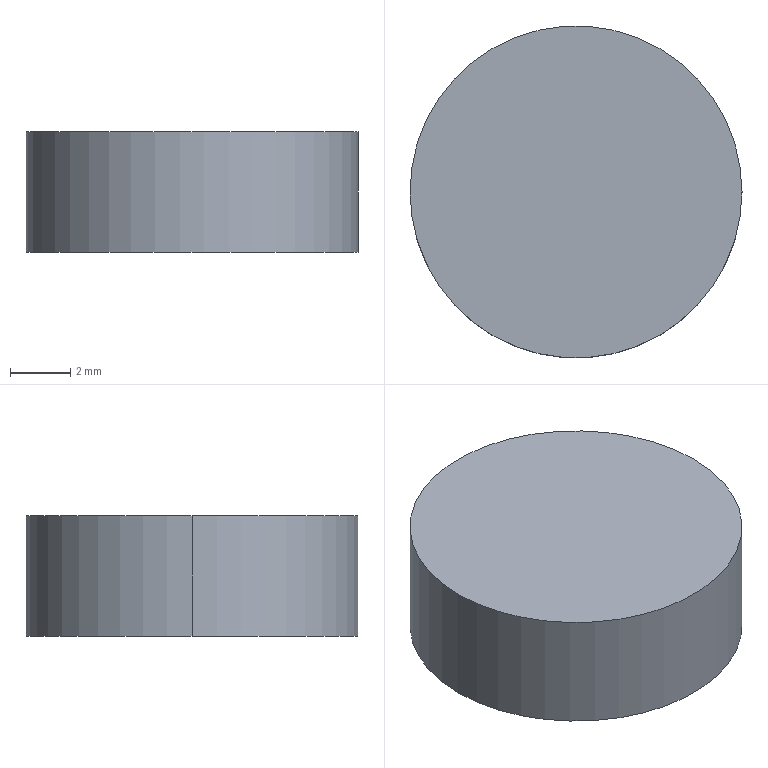Part | STEP file | 1_id258_x_t | 1 solid | 4 faces | box 11 x 11 x 4 mm | volume 380.137 mm3 | plane 2 | cylinder 2 | commonest cylinder face diameters 11 x2
STEP:
#1=CARTESIAN_POINT('',(0.,0.,0.));
#2=DIRECTION('',(0.,0.,1.));
#3=DIRECTION('',(1.,0.,0.));
#4=AXIS2_PLACEMENT_3D('',#1,#2,#3);
#5=CARTESIAN_POINT('',(201.65,177.5,39.075));
#6=VERTEX_POINT('',#5);
#7=CARTESIAN_POINT('',(212.65,177.5,39.075));
#8=VERTEX_POINT('',#7);
#9=CARTESIAN_POINT('',(207.15,177.5,39.075));
#10=DIRECTION('',(0.,0.,1.));
#11=DIRECTION('',(-1.,0.,0.));
#12=AXIS2_PLACEMENT_3D('',#9,#10,#11);
#13=CIRCLE('',#12,5.5);
#14=CARTESIAN_POINT('',(274.812,177.5,39.075));
#15=DIRECTION('',(0.,0.,-1.));
#16=DIRECTION('',(-1.,0.,0.));
#17=AXIS2_PLACEMENT_3D('',#14,#15,#16);
#18=PLANE('',#17);
#19=CARTESIAN_POINT('',(73.162,0.));
#20=CARTESIAN_POINT('',(73.162,-9.526));
#21=CARTESIAN_POINT('',(64.912,-4.763));
#22=CARTESIAN_POINT('',(56.663,0.));
#23=CARTESIAN_POINT('',(64.912,4.763));
#24=CARTESIAN_POINT('',(73.162,9.526));
#25=CARTESIAN_POINT('',(73.162,0.));
#26=(BOUNDED_CURVE()B_SPLINE_CURVE(2,(#19,#20,#21,#22,#23,#24,#25),.UNSPECIFIED.,.T.,.F.)B_SPLINE_CURVE_WITH_KNOTS((1,2,2,2,2,1),(-2.094,0.,2.094,4.189,6.283,8.378),.UNSPECIFIED.)CURVE()GEOMETRIC_REPRESENTATION_ITEM()RATIONAL_B_SPLINE_CURVE((1.,0.5,1.,0.5,1.,0.5,1.))REPRESENTATION_ITEM(''));
#27=(GEOMETRIC_REPRESENTATION_CONTEXT(2)PARAMETRIC_REPRESENTATION_CONTEXT()REPRESENTATION_CONTEXT('',''));
#28=DEFINITIONAL_REPRESENTATION('',(#26),#27);
#29=PCURVE('',#18,#28);
#30=CARTESIAN_POINT('',(207.15,177.5,43.075));
#31=DIRECTION('',(0.,0.,-1.));
#32=DIRECTION('',(-1.,0.,0.));
#33=AXIS2_PLACEMENT_3D('',#30,#31,#32);
#34=CYLINDRICAL_SURFACE('',#33,5.5);
#35=CARTESIAN_POINT('',(6.283,4.));
#36=DIRECTION('',(-1.,0.));
#37=VECTOR('',#36,1.);
#38=LINE('',#35,#37);
#39=(GEOMETRIC_REPRESENTATION_CONTEXT(2)PARAMETRIC_REPRESENTATION_CONTEXT()REPRESENTATION_CONTEXT('',''));
#40=DEFINITIONAL_REPRESENTATION('',(#38),#39);
#41=PCURVE('',#34,#40);
#42=SURFACE_CURVE('',#13,(#29,#41),.PCURVE_S1.);
#43=EDGE_CURVE('',#6,#8,#42,.T.);
#44=ORIENTED_EDGE('',*,*,#43,.F.);
#45=CARTESIAN_POINT('',(207.15,177.5,39.075));
#46=DIRECTION('',(0.,0.,1.));
#47=DIRECTION('',(-1.,0.,0.));
#48=AXIS2_PLACEMENT_3D('',#45,#46,#47);
#49=CIRCLE('',#48,5.5);
#50=CARTESIAN_POINT('',(73.162,0.));
#51=CARTESIAN_POINT('',(73.162,-9.526));
#52=CARTESIAN_POINT('',(64.912,-4.763));
#53=CARTESIAN_POINT('',(56.663,0.));
#54=CARTESIAN_POINT('',(64.912,4.763));
#55=CARTESIAN_POINT('',(73.162,9.526));
#56=CARTESIAN_POINT('',(73.162,0.));
#57=(BOUNDED_CURVE()B_SPLINE_CURVE(2,(#50,#51,#52,#53,#54,#55,#56),.UNSPECIFIED.,.T.,.F.)B_SPLINE_CURVE_WITH_KNOTS((1,2,2,2,2,1),(-2.094,0.,2.094,4.189,6.283,8.378),.UNSPECIFIED.)CURVE()GEOMETRIC_REPRESENTATION_ITEM()RATIONAL_B_SPLINE_CURVE((1.,0.5,1.,0.5,1.,0.5,1.))REPRESENTATION_ITEM(''));
#58=(GEOMETRIC_REPRESENTATION_CONTEXT(2)PARAMETRIC_REPRESENTATION_CONTEXT()REPRESENTATION_CONTEXT('',''));
#59=DEFINITIONAL_REPRESENTATION('',(#57),#58);
#60=PCURVE('',#18,#59);
#61=CARTESIAN_POINT('',(207.15,177.5,43.075));
#62=DIRECTION('',(0.,0.,-1.));
#63=DIRECTION('',(-1.,0.,0.));
#64=AXIS2_PLACEMENT_3D('',#61,#62,#63);
#65=CYLINDRICAL_SURFACE('',#64,5.5);
#66=CARTESIAN_POINT('',(6.283,4.));
#67=DIRECTION('',(-1.,0.));
#68=VECTOR('',#67,1.);
#69=LINE('',#66,#68);
#70=(GEOMETRIC_REPRESENTATION_CONTEXT(2)PARAMETRIC_REPRESENTATION_CONTEXT()REPRESENTATION_CONTEXT('',''));
#71=DEFINITIONAL_REPRESENTATION('',(#69),#70);
#72=PCURVE('',#65,#71);
#73=SURFACE_CURVE('',#49,(#60,#72),.PCURVE_S1.);
#74=EDGE_CURVE('',#8,#6,#73,.T.);
#75=ORIENTED_EDGE('',*,*,#74,.F.);
#76=EDGE_LOOP('',(#44,#75));
#77=FACE_BOUND('',#76,.T.);
#78=ADVANCED_FACE('',(#77),#18,.T.);
#79=CARTESIAN_POINT('',(201.65,177.5,43.075));
#80=VERTEX_POINT('',#79);
#81=CARTESIAN_POINT('',(212.65,177.5,43.075));
#82=VERTEX_POINT('',#81);
#83=CARTESIAN_POINT('',(207.15,177.5,43.075));
#84=DIRECTION('',(0.,0.,1.));
#85=DIRECTION('',(-1.,0.,0.));
#86=AXIS2_PLACEMENT_3D('',#83,#84,#85);
#87=CIRCLE('',#86,5.5);
#88=CARTESIAN_POINT('',(207.15,177.5,43.075));
#89=DIRECTION('',(0.,0.,1.));
#90=DIRECTION('',(1.,0.,0.));
#91=AXIS2_PLACEMENT_3D('',#88,#89,#90);
#92=PLANE('',#91);
#93=CARTESIAN_POINT('',(0.,0.));
#94=DIRECTION('',(-1.,0.));
#95=AXIS2_PLACEMENT_2D('',#93,#94);
#96=CIRCLE('',#95,5.5);
#97=(GEOMETRIC_REPRESENTATION_CONTEXT(2)PARAMETRIC_REPRESENTATION_CONTEXT()REPRESENTATION_CONTEXT('',''));
#98=DEFINITIONAL_REPRESENTATION('',(#96),#97);
#99=PCURVE('',#92,#98);
#100=CARTESIAN_POINT('',(6.283,0.));
#101=DIRECTION('',(-1.,0.));
#102=VECTOR('',#101,1.);
#103=LINE('',#100,#102);
#104=(GEOMETRIC_REPRESENTATION_CONTEXT(2)PARAMETRIC_REPRESENTATION_CONTEXT()REPRESENTATION_CONTEXT('',''));
#105=DEFINITIONAL_REPRESENTATION('',(#103),#104);
#106=PCURVE('',#34,#105);
#107=SURFACE_CURVE('',#87,(#99,#106),.PCURVE_S1.);
#108=EDGE_CURVE('',#80,#82,#107,.T.);
#109=ORIENTED_EDGE('',*,*,#108,.T.);
#110=CARTESIAN_POINT('',(207.15,177.5,43.075));
#111=DIRECTION('',(0.,0.,1.));
#112=DIRECTION('',(1.,0.,0.));
#113=AXIS2_PLACEMENT_3D('',#110,#111,#112);
#114=CIRCLE('',#113,5.5);
#115=CARTESIAN_POINT('',(0.,0.));
#116=DIRECTION('',(1.,0.));
#117=AXIS2_PLACEMENT_2D('',#115,#116);
#118=CIRCLE('',#117,5.5);
#119=(GEOMETRIC_REPRESENTATION_CONTEXT(2)PARAMETRIC_REPRESENTATION_CONTEXT()REPRESENTATION_CONTEXT('',''));
#120=DEFINITIONAL_REPRESENTATION('',(#118),#119);
#121=PCURVE('',#92,#120);
#122=CARTESIAN_POINT('',(3.142,0.));
#123=DIRECTION('',(-1.,0.));
#124=VECTOR('',#123,1.);
#125=LINE('',#122,#124);
#126=(GEOMETRIC_REPRESENTATION_CONTEXT(2)PARAMETRIC_REPRESENTATION_CONTEXT()REPRESENTATION_CONTEXT('',''));
#127=DEFINITIONAL_REPRESENTATION('',(#125),#126);
#128=PCURVE('',#65,#127);
#129=SURFACE_CURVE('',#114,(#121,#128),.PCURVE_S1.);
#130=EDGE_CURVE('',#82,#80,#129,.T.);
#131=ORIENTED_EDGE('',*,*,#130,.T.);
#132=EDGE_LOOP('',(#109,#131));
#133=FACE_BOUND('',#132,.T.);
#134=ADVANCED_FACE('',(#133),#92,.T.);
#135=CARTESIAN_POINT('',(212.65,177.5,43.075));
#136=DIRECTION('',(0.,0.,1.));
#137=VECTOR('',#136,1.);
#138=LINE('',#135,#137);
#139=CARTESIAN_POINT('',(3.142,0.));
#140=DIRECTION('',(0.,-1.));
#141=VECTOR('',#140,1.);
#142=LINE('',#139,#141);
#143=(GEOMETRIC_REPRESENTATION_CONTEXT(2)PARAMETRIC_REPRESENTATION_CONTEXT()REPRESENTATION_CONTEXT('',''));
#144=DEFINITIONAL_REPRESENTATION('',(#142),#143);
#145=PCURVE('',#65,#144);
#146=CARTESIAN_POINT('',(3.142,0.));
#147=DIRECTION('',(0.,-1.));
#148=VECTOR('',#147,1.);
#149=LINE('',#146,#148);
#150=(GEOMETRIC_REPRESENTATION_CONTEXT(2)PARAMETRIC_REPRESENTATION_CONTEXT()REPRESENTATION_CONTEXT('',''));
#151=DEFINITIONAL_REPRESENTATION('',(#149),#150);
#152=PCURVE('',#34,#151);
#153=SURFACE_CURVE('',#138,(#145,#152),.PCURVE_S1.);
#154=EDGE_CURVE('',#8,#82,#153,.T.);
#155=ORIENTED_EDGE('',*,*,#154,.F.);
#156=ORIENTED_EDGE('',*,*,#74,.T.);
#157=CARTESIAN_POINT('',(201.65,177.5,43.075));
#158=DIRECTION('',(0.,0.,-1.));
#159=VECTOR('',#158,1.);
#160=LINE('',#157,#159);
#161=CARTESIAN_POINT('',(0.,0.));
#162=DIRECTION('',(0.,1.));
#163=VECTOR('',#162,1.);
#164=LINE('',#161,#163);
#165=(GEOMETRIC_REPRESENTATION_CONTEXT(2)PARAMETRIC_REPRESENTATION_CONTEXT()REPRESENTATION_CONTEXT('',''));
#166=DEFINITIONAL_REPRESENTATION('',(#164),#165);
#167=PCURVE('',#65,#166);
#168=CARTESIAN_POINT('',(6.283,0.));
#169=DIRECTION('',(0.,1.));
#170=VECTOR('',#169,1.);
#171=LINE('',#168,#170);
#172=(GEOMETRIC_REPRESENTATION_CONTEXT(2)PARAMETRIC_REPRESENTATION_CONTEXT()REPRESENTATION_CONTEXT('',''));
#173=DEFINITIONAL_REPRESENTATION('',(#171),#172);
#174=PCURVE('',#34,#173);
#175=SURFACE_CURVE('',#160,(#167,#174),.PCURVE_S1.);
#176=EDGE_CURVE('',#80,#6,#175,.T.);
#177=ORIENTED_EDGE('',*,*,#176,.F.);
#178=ORIENTED_EDGE('',*,*,#130,.F.);
#179=EDGE_LOOP('',(#155,#156,#177,#178));
#180=FACE_BOUND('',#179,.T.);
#181=ADVANCED_FACE('',(#180),#65,.T.);
#182=ORIENTED_EDGE('',*,*,#176,.T.);
#183=ORIENTED_EDGE('',*,*,#43,.T.);
#184=ORIENTED_EDGE('',*,*,#154,.T.);
#185=ORIENTED_EDGE('',*,*,#108,.F.);
#186=EDGE_LOOP('',(#182,#183,#184,#185));
#187=FACE_BOUND('',#186,.T.);
#188=ADVANCED_FACE('',(#187),#34,.T.);
#189=CLOSED_SHELL('',(#78,#134,#181,#188));
#190=MANIFOLD_SOLID_BREP('',#189);
#191=(LENGTH_UNIT()NAMED_UNIT(*)SI_UNIT(.MILLI.,.METRE.));
#192=UNCERTAINTY_MEASURE_WITH_UNIT(LENGTH_MEASURE(0.0000001),#191,'','');
#193=(NAMED_UNIT(*)PLANE_ANGLE_UNIT()SI_UNIT($,.RADIAN.));
#194=(NAMED_UNIT(*)SI_UNIT($,.STERADIAN.)SOLID_ANGLE_UNIT());
#195=(GEOMETRIC_REPRESENTATION_CONTEXT(3)GLOBAL_UNCERTAINTY_ASSIGNED_CONTEXT((#192))GLOBAL_UNIT_ASSIGNED_CONTEXT((#191,#193,#194))REPRESENTATION_CONTEXT('',''));
#196=ADVANCED_BREP_SHAPE_REPRESENTATION('',(#4,#190),#195);